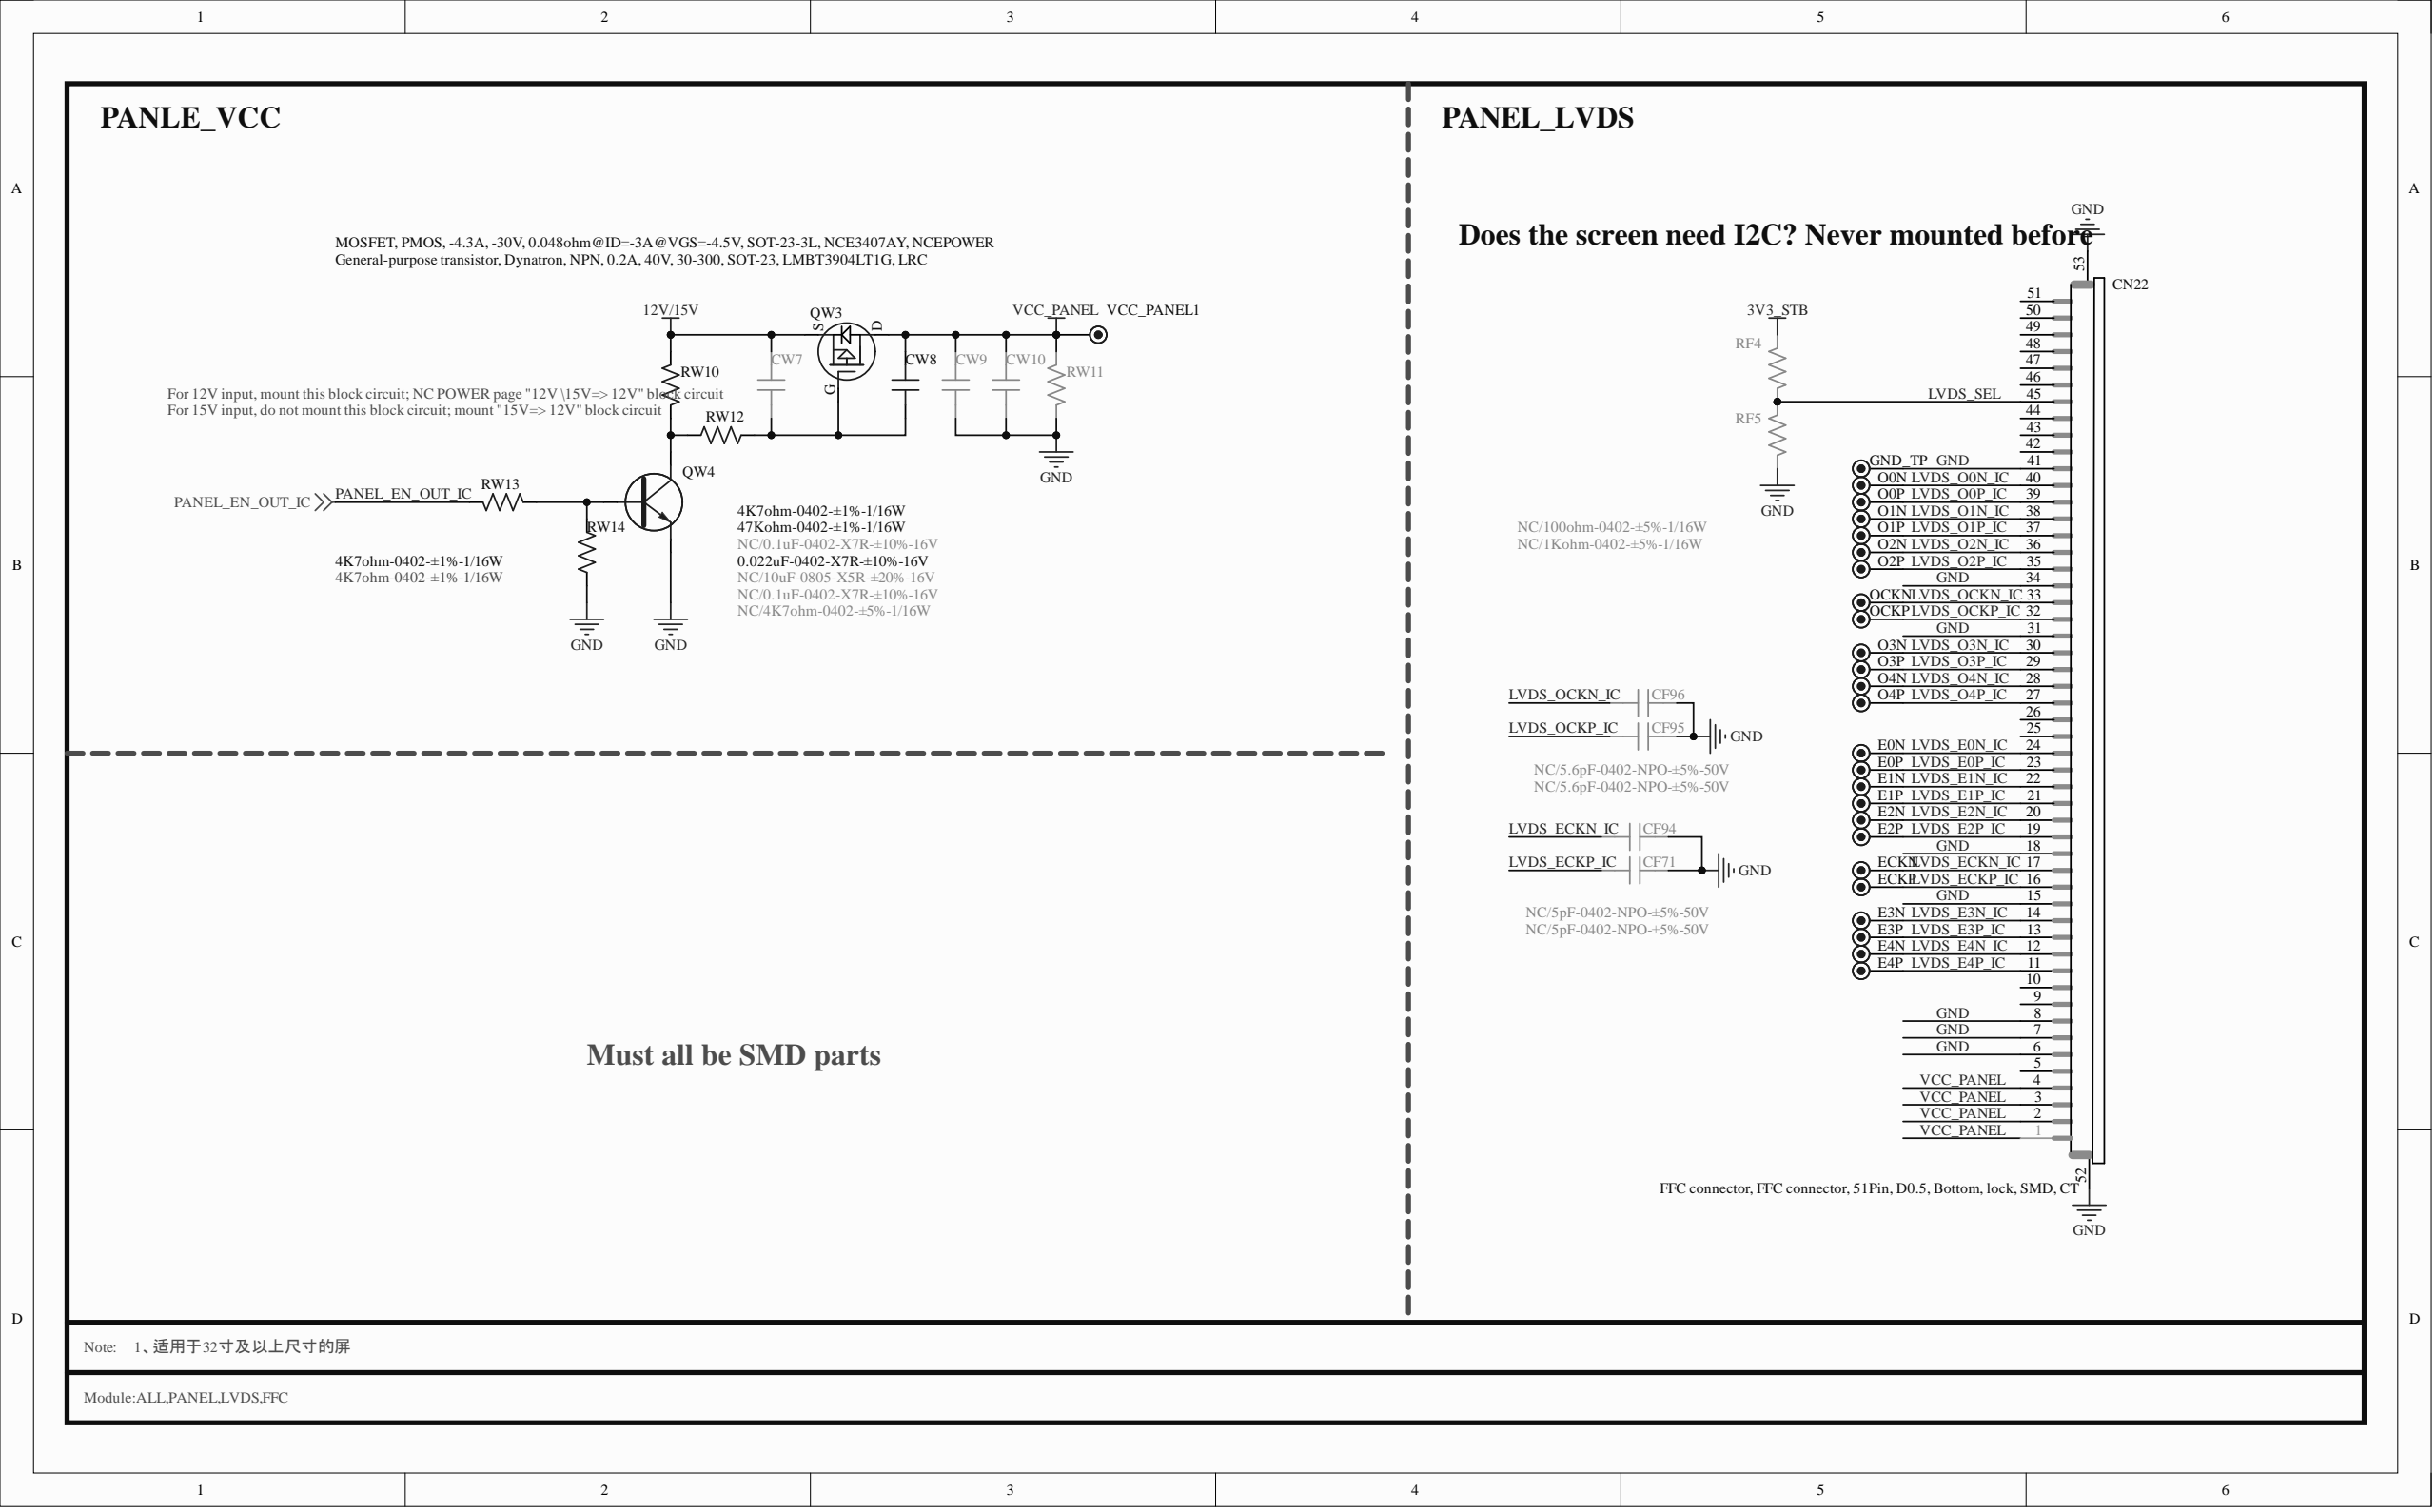Circuit board | Altium Designer | 541 parts | 263 nets | one sheet of the schematic
Parts on this sheet (reference | value | footprint):
CF71 | NC/5pF-0402-NPO-±5%-50V | C0402
CF94 | NC/5pF-0402-NPO-±5%-50V | C0402
CF95 | NC/5.6pF-0402-NPO-±5%-50V | C0402
CF96 | NC/5.6pF-0402-NPO-±5%-50V | C0402
CN22 | FFC connector, FFC connector, 51Pin, D0.5, Bottom, lock, SMD, CT | FFC51H/0.5S-8
CW7 | NC/0.1uF-0402-X7R-±10%-16V | C0402
CW8 | 0.022uF-0402-X7R-±10%-16V | C0402
CW9 | NC/10uF-0805-X5R-±20%-16V | C0805
CW10 | NC/0.1uF-0402-X7R-±10%-16V | C0402
E0N | TEST | TP
E0P | TEST | TP
E1N | TEST | TP
E1P | TEST | TP
E2N | TEST | TP
E2P | TEST | TP
E3N | TEST | TP
E3P | TEST | TP
E4N | TEST | TP
E4P | TEST | TP
ECKN | TEST | TP
ECKP | TEST | TP
GND_TP | TEST | TP
O0N | TEST | TP
O0P | TEST | TP
O1N | TEST | TP
O1P | TEST | TP
O2N | TEST | TP
O2P | TEST | TP
O3N | TEST | TP
O3P | TEST | TP
O4N | TEST | TP
O4P | TEST | TP
OCKN | TEST | TP
OCKP | TEST | TP
QW3 | MOSFET, PMOS, -4.3A, -30V, 0.048ohm@ID=-3A@VGS=-4.5V, SOT-23-3L, NCE3407AY, NCEPOWER | SOT-23-1
QW4 | General-purpose transistor, Dynatron, NPN, 0.2A, 40V, 30-300, SOT-23, LMBT3904LT1G, LRC | SOT-23
RF4 | NC/100ohm-0402-±5%-1/16W | R0402
RF5 | NC/1Kohm-0402-±5%-1/16W | R0402
RW10 | 4K7ohm-0402-±1%-1/16W | R0402
RW11 | NC/4K7ohm-0402-±5%-1/16W | R0402
RW12 | 47Kohm-0402-±1%-1/16W | R0402
RW13 | 4K7ohm-0402-±1%-1/16W | R0402
RW14 | 4K7ohm-0402-±1%-1/16W | R0402
VCC_PANEL1 | TEST | TP
Nets of these parts (net: part-pin ...):
VCC_PANEL: CW8-1 CW9-2 CW10-2 QW3-D RW11-2 VCC_PANEL1-1 CN22-1 CN22-2 CN22-3 CN22-4
PANEL_EN_OUT_IC: RW13-1
NetQW4_C: QW4-C RW10-1 RW12-1
NetQW4_B: QW4-B RW13-2 RW14-1
NetCW7_1: CW7-1 CW8-2 QW3-G RW12-2
LVDS_SEL: RF4-1 RF5-2 CN22-45
LVDS_OCKP_IC: CF95-2 OCKP-1 CN22-32
LVDS_OCKN_IC: CF96-2 OCKN-1 CN22-33
LVDS_O4P_IC: O4P-1 CN22-27
LVDS_O4N_IC: O4N-1 CN22-28
LVDS_O3P_IC: O3P-1 CN22-29
LVDS_O3N_IC: O3N-1 CN22-30
LVDS_O2P_IC: O2P-1 CN22-35
LVDS_O2N_IC: O2N-1 CN22-36
LVDS_O1P_IC: O1P-1 CN22-37
LVDS_O1N_IC: O1N-1 CN22-38
LVDS_O0P_IC: O0P-1 CN22-39
LVDS_O0N_IC: O0N-1 CN22-40
LVDS_ECKP_IC: CF71-2 ECKP-1 CN22-16
LVDS_ECKN_IC: CF94-2 ECKN-1 CN22-17
LVDS_E4P_IC: E4P-1 CN22-11
LVDS_E4N_IC: E4N-1 CN22-12
LVDS_E3P_IC: E3P-1 CN22-13
LVDS_E3N_IC: E3N-1 CN22-14
LVDS_E2P_IC: E2P-1 CN22-19
LVDS_E2N_IC: E2N-1 CN22-20
LVDS_E1P_IC: E1P-1 CN22-21
LVDS_E1N_IC: E1N-1 CN22-22
LVDS_E0P_IC: E0P-1 CN22-23
LVDS_E0N_IC: E0N-1 CN22-24
GND: CF71-1 CF94-1 CF95-1 CF96-1 CW9-1 CW10-1 GND_TP-1 QW4-E RF5-1 RW11-1 RW14-2 CN22-6 CN22-7 CN22-8 CN22-15 CN22-18 CN22-31 CN22-34 CN22-41 CN22-52 CN22-53
12V/15V: CW7-2 QW3-S RW10-2
3V3_STB: RF4-2